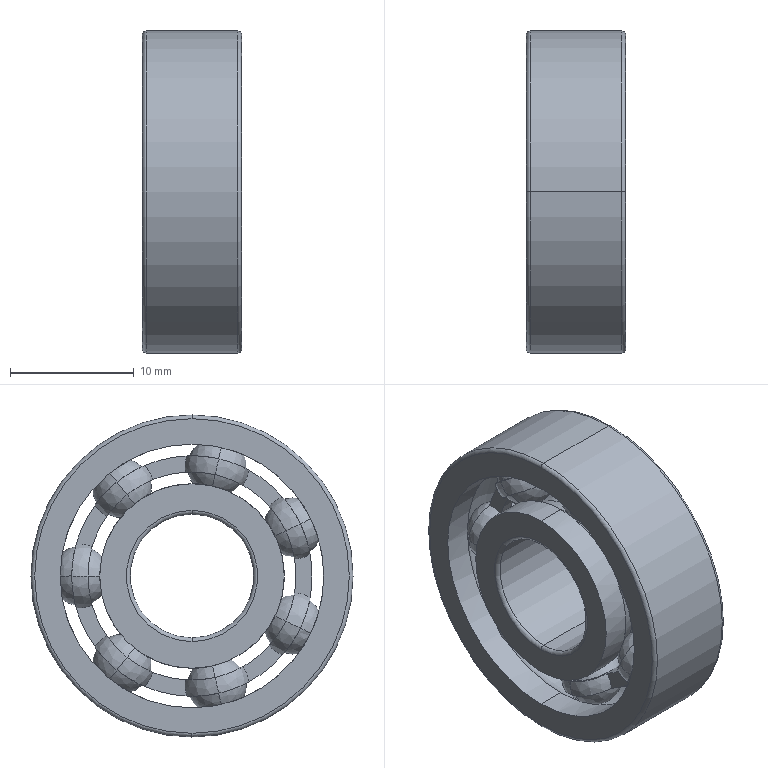Part | NX | features BREP 1 | 1 solid | 122 faces | box 8 x 26 x 26 mm | volume 2406 mm3 | sphere 56 | torus 32 | plane 18 | cylinder 16 | commonest cylinder face diameters 14.9 x4 21.3 x4 10 x2 16.79 x2 19.41 x2 26 x2